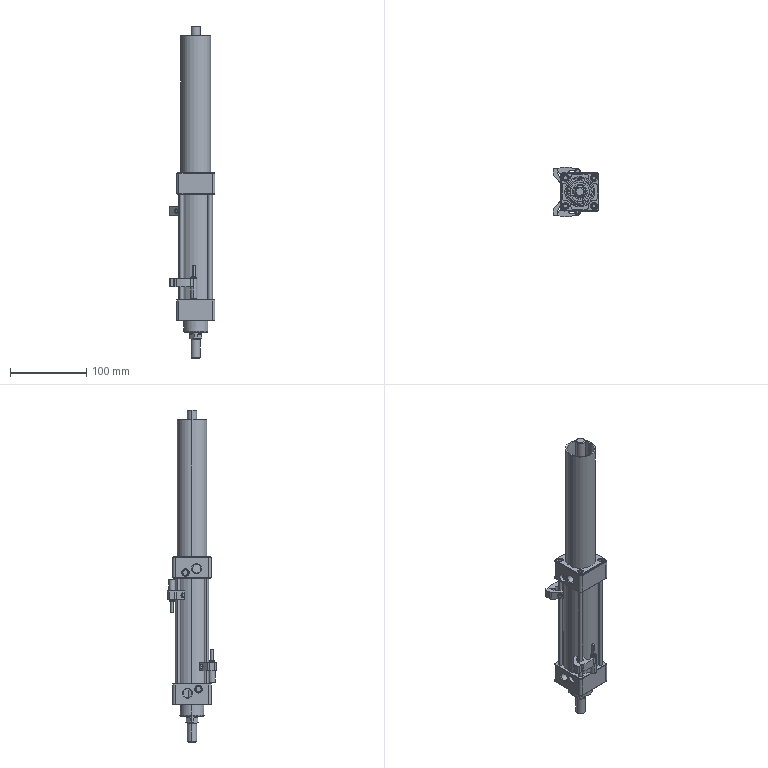Part | SolidWorks | 14 solids | 891 faces | box 59.782 x 64.739 x 435 mm | volume 326240 mm3 | plane 390 | cylinder 309 | cone 132 | torus 60 | commonest cylinder face diameters 6 x56 2 x26 4.917 x16 6.5 x16 9 x16 9.5 x16